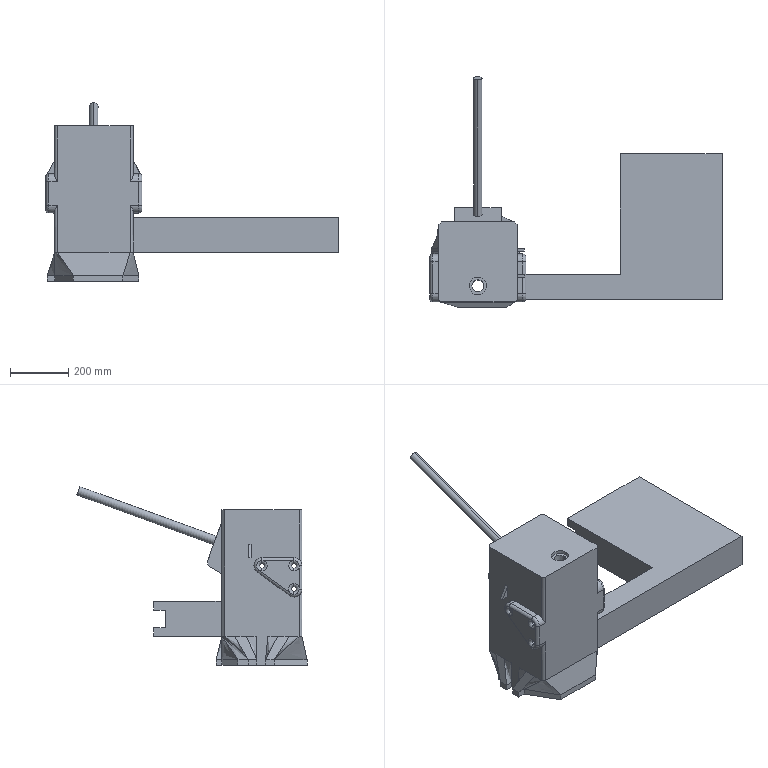Part | SolidWorks | 1 solid | 127 faces | box 1005 x 791.422 x 614.545 mm | volume 64772988 mm3 | plane 65 | cylinder 32 | torus 19 | spline 11 | commonest cylinder face diameters 20 x10 55 x7 16 x6 60 x4 30 x2 41 x2